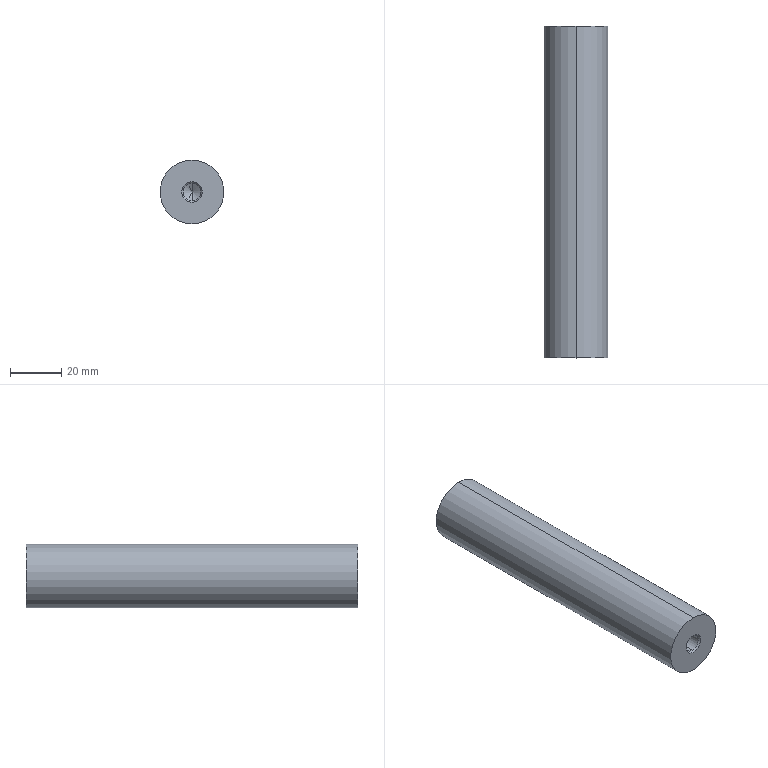Part | STEP file | A14-032 | 1 solid | 16 faces | box 25 x 130 x 25 mm | volume 62139 mm3 | cone 8 | cylinder 6 | plane 2 | commonest cylinder face diameters 6.8 x4 25 x2
STEP:
#1=CARTESIAN_POINT('',(0.,0.,0.));
#2=DIRECTION('',(0.,0.,1.));
#3=DIRECTION('',(1.,0.,0.));
#4=AXIS2_PLACEMENT_3D('',#1,#2,#3);
#5=CARTESIAN_POINT('',(0.,64.375,3.4));
#6=VERTEX_POINT('',#5);
#7=CARTESIAN_POINT('',(0.,65.,4.025));
#8=VERTEX_POINT('',#7);
#9=CARTESIAN_POINT('',(0.,65.,4.025));
#10=DIRECTION('',(0.,0.7071,0.7071));
#11=VECTOR('',#10,1.);
#12=LINE('',#9,#11);
#13=CARTESIAN_POINT('',(0.,65.,0.));
#14=DIRECTION('',(0.,1.,0.));
#15=DIRECTION('',(0.,0.,1.));
#16=AXIS2_PLACEMENT_3D('',#13,#14,#15);
#17=CONICAL_SURFACE('',#16,4.025,0.7854);
#18=CARTESIAN_POINT('',(6.283,0.));
#19=DIRECTION('',(0.,1.));
#20=VECTOR('',#19,1.);
#21=LINE('',#18,#20);
#22=(GEOMETRIC_REPRESENTATION_CONTEXT(2)PARAMETRIC_REPRESENTATION_CONTEXT()REPRESENTATION_CONTEXT('',''));
#23=DEFINITIONAL_REPRESENTATION('',(#21),#22);
#24=PCURVE('',#17,#23);
#25=CARTESIAN_POINT('',(0.,65.,0.));
#26=DIRECTION('',(0.,1.,0.));
#27=DIRECTION('',(0.,0.,1.));
#28=AXIS2_PLACEMENT_3D('',#25,#26,#27);
#29=CONICAL_SURFACE('',#28,4.025,0.7854);
#30=CARTESIAN_POINT('',(0.,0.));
#31=DIRECTION('',(0.,1.));
#32=VECTOR('',#31,1.);
#33=LINE('',#30,#32);
#34=(GEOMETRIC_REPRESENTATION_CONTEXT(2)PARAMETRIC_REPRESENTATION_CONTEXT()REPRESENTATION_CONTEXT('',''));
#35=DEFINITIONAL_REPRESENTATION('',(#33),#34);
#36=PCURVE('',#29,#35);
#37=SURFACE_CURVE('',#12,(#24,#36),.PCURVE_S1.);
#38=EDGE_CURVE('',#6,#8,#37,.T.);
#39=ORIENTED_EDGE('',*,*,#38,.T.);
#40=CARTESIAN_POINT('',(0.,65.,-4.025));
#41=VERTEX_POINT('',#40);
#42=CARTESIAN_POINT('',(0.,65.,0.));
#43=DIRECTION('',(0.,1.,0.));
#44=DIRECTION('',(0.,0.,1.));
#45=AXIS2_PLACEMENT_3D('',#42,#43,#44);
#46=CIRCLE('',#45,4.025);
#47=CARTESIAN_POINT('',(0.,0.));
#48=DIRECTION('',(1.,0.));
#49=VECTOR('',#48,1.);
#50=LINE('',#47,#49);
#51=(GEOMETRIC_REPRESENTATION_CONTEXT(2)PARAMETRIC_REPRESENTATION_CONTEXT()REPRESENTATION_CONTEXT('',''));
#52=DEFINITIONAL_REPRESENTATION('',(#50),#51);
#53=PCURVE('',#17,#52);
#54=CARTESIAN_POINT('',(0.,65.,0.));
#55=DIRECTION('',(0.,1.,0.));
#56=DIRECTION('',(0.,0.,1.));
#57=AXIS2_PLACEMENT_3D('',#54,#55,#56);
#58=PLANE('',#57);
#59=CARTESIAN_POINT('',(0.,0.));
#60=DIRECTION('',(1.,0.));
#61=AXIS2_PLACEMENT_2D('',#59,#60);
#62=CIRCLE('',#61,4.025);
#63=(GEOMETRIC_REPRESENTATION_CONTEXT(2)PARAMETRIC_REPRESENTATION_CONTEXT()REPRESENTATION_CONTEXT('',''));
#64=DEFINITIONAL_REPRESENTATION('',(#62),#63);
#65=PCURVE('',#58,#64);
#66=SURFACE_CURVE('',#46,(#53,#65),.PCURVE_S1.);
#67=EDGE_CURVE('',#41,#8,#66,.T.);
#68=ORIENTED_EDGE('',*,*,#67,.F.);
#69=CARTESIAN_POINT('',(0.,64.375,-3.4));
#70=VERTEX_POINT('',#69);
#71=CARTESIAN_POINT('',(0.,65.,-4.025));
#72=DIRECTION('',(0.,0.7071,-0.7071));
#73=VECTOR('',#72,1.);
#74=LINE('',#71,#73);
#75=CARTESIAN_POINT('',(3.142,0.));
#76=DIRECTION('',(0.,1.));
#77=VECTOR('',#76,1.);
#78=LINE('',#75,#77);
#79=(GEOMETRIC_REPRESENTATION_CONTEXT(2)PARAMETRIC_REPRESENTATION_CONTEXT()REPRESENTATION_CONTEXT('',''));
#80=DEFINITIONAL_REPRESENTATION('',(#78),#79);
#81=PCURVE('',#17,#80);
#82=CARTESIAN_POINT('',(3.142,0.));
#83=DIRECTION('',(0.,1.));
#84=VECTOR('',#83,1.);
#85=LINE('',#82,#84);
#86=(GEOMETRIC_REPRESENTATION_CONTEXT(2)PARAMETRIC_REPRESENTATION_CONTEXT()REPRESENTATION_CONTEXT('',''));
#87=DEFINITIONAL_REPRESENTATION('',(#85),#86);
#88=PCURVE('',#29,#87);
#89=SURFACE_CURVE('',#74,(#81,#88),.PCURVE_S1.);
#90=EDGE_CURVE('',#70,#41,#89,.T.);
#91=ORIENTED_EDGE('',*,*,#90,.F.);
#92=CARTESIAN_POINT('',(0.,64.375,0.));
#93=DIRECTION('',(0.,1.,0.));
#94=DIRECTION('',(0.,0.,1.));
#95=AXIS2_PLACEMENT_3D('',#92,#93,#94);
#96=CIRCLE('',#95,3.4);
#97=CARTESIAN_POINT('',(0.,-0.625));
#98=DIRECTION('',(1.,0.));
#99=VECTOR('',#98,1.);
#100=LINE('',#97,#99);
#101=(GEOMETRIC_REPRESENTATION_CONTEXT(2)PARAMETRIC_REPRESENTATION_CONTEXT()REPRESENTATION_CONTEXT('',''));
#102=DEFINITIONAL_REPRESENTATION('',(#100),#101);
#103=PCURVE('',#17,#102);
#104=CARTESIAN_POINT('',(0.,65.,0.));
#105=DIRECTION('',(0.,1.,0.));
#106=DIRECTION('',(0.,0.,1.));
#107=AXIS2_PLACEMENT_3D('',#104,#105,#106);
#108=CYLINDRICAL_SURFACE('',#107,3.4);
#109=CARTESIAN_POINT('',(0.,-0.625));
#110=DIRECTION('',(1.,0.));
#111=VECTOR('',#110,1.);
#112=LINE('',#109,#111);
#113=(GEOMETRIC_REPRESENTATION_CONTEXT(2)PARAMETRIC_REPRESENTATION_CONTEXT()REPRESENTATION_CONTEXT('',''));
#114=DEFINITIONAL_REPRESENTATION('',(#112),#113);
#115=PCURVE('',#108,#114);
#116=SURFACE_CURVE('',#96,(#103,#115),.PCURVE_S1.);
#117=EDGE_CURVE('',#70,#6,#116,.T.);
#118=ORIENTED_EDGE('',*,*,#117,.T.);
#119=EDGE_LOOP('',(#39,#68,#91,#118));
#120=FACE_BOUND('',#119,.F.);
#121=ADVANCED_FACE('',(#120),#17,.F.);
#122=CARTESIAN_POINT('',(0.,42.75,3.4));
#123=VERTEX_POINT('',#122);
#124=CARTESIAN_POINT('',(0.,65.,3.4));
#125=DIRECTION('',(0.,1.,0.));
#126=VECTOR('',#125,1.);
#127=LINE('',#124,#126);
#128=CARTESIAN_POINT('',(6.283,0.));
#129=DIRECTION('',(0.,1.));
#130=VECTOR('',#129,1.);
#131=LINE('',#128,#130);
#132=(GEOMETRIC_REPRESENTATION_CONTEXT(2)PARAMETRIC_REPRESENTATION_CONTEXT()REPRESENTATION_CONTEXT('',''));
#133=DEFINITIONAL_REPRESENTATION('',(#131),#132);
#134=PCURVE('',#108,#133);
#135=CARTESIAN_POINT('',(0.,65.,0.));
#136=DIRECTION('',(0.,1.,0.));
#137=DIRECTION('',(0.,0.,1.));
#138=AXIS2_PLACEMENT_3D('',#135,#136,#137);
#139=CYLINDRICAL_SURFACE('',#138,3.4);
#140=CARTESIAN_POINT('',(0.,0.));
#141=DIRECTION('',(0.,1.));
#142=VECTOR('',#141,1.);
#143=LINE('',#140,#142);
#144=(GEOMETRIC_REPRESENTATION_CONTEXT(2)PARAMETRIC_REPRESENTATION_CONTEXT()REPRESENTATION_CONTEXT('',''));
#145=DEFINITIONAL_REPRESENTATION('',(#143),#144);
#146=PCURVE('',#139,#145);
#147=SURFACE_CURVE('',#127,(#134,#146),.PCURVE_S1.);
#148=EDGE_CURVE('',#123,#6,#147,.T.);
#149=ORIENTED_EDGE('',*,*,#148,.T.);
#150=ORIENTED_EDGE('',*,*,#117,.F.);
#151=CARTESIAN_POINT('',(0.,42.75,-3.4));
#152=VERTEX_POINT('',#151);
#153=CARTESIAN_POINT('',(0.,65.,-3.4));
#154=DIRECTION('',(0.,1.,0.));
#155=VECTOR('',#154,1.);
#156=LINE('',#153,#155);
#157=CARTESIAN_POINT('',(3.142,0.));
#158=DIRECTION('',(0.,1.));
#159=VECTOR('',#158,1.);
#160=LINE('',#157,#159);
#161=(GEOMETRIC_REPRESENTATION_CONTEXT(2)PARAMETRIC_REPRESENTATION_CONTEXT()REPRESENTATION_CONTEXT('',''));
#162=DEFINITIONAL_REPRESENTATION('',(#160),#161);
#163=PCURVE('',#108,#162);
#164=CARTESIAN_POINT('',(3.142,0.));
#165=DIRECTION('',(0.,1.));
#166=VECTOR('',#165,1.);
#167=LINE('',#164,#166);
#168=(GEOMETRIC_REPRESENTATION_CONTEXT(2)PARAMETRIC_REPRESENTATION_CONTEXT()REPRESENTATION_CONTEXT('',''));
#169=DEFINITIONAL_REPRESENTATION('',(#167),#168);
#170=PCURVE('',#139,#169);
#171=SURFACE_CURVE('',#156,(#163,#170),.PCURVE_S1.);
#172=EDGE_CURVE('',#152,#70,#171,.T.);
#173=ORIENTED_EDGE('',*,*,#172,.F.);
#174=CARTESIAN_POINT('',(0.,42.75,0.));
#175=DIRECTION('',(0.,1.,0.));
#176=DIRECTION('',(0.,0.,1.));
#177=AXIS2_PLACEMENT_3D('',#174,#175,#176);
#178=CIRCLE('',#177,3.4);
#179=CARTESIAN_POINT('',(0.,-22.25));
#180=DIRECTION('',(1.,0.));
#181=VECTOR('',#180,1.);
#182=LINE('',#179,#181);
#183=(GEOMETRIC_REPRESENTATION_CONTEXT(2)PARAMETRIC_REPRESENTATION_CONTEXT()REPRESENTATION_CONTEXT('',''));
#184=DEFINITIONAL_REPRESENTATION('',(#182),#183);
#185=PCURVE('',#108,#184);
#186=CARTESIAN_POINT('',(0.,42.75,0.));
#187=DIRECTION('',(0.,1.,0.));
#188=DIRECTION('',(0.,0.,1.));
#189=AXIS2_PLACEMENT_3D('',#186,#187,#188);
#190=CONICAL_SURFACE('',#189,3.4,1.03);
#191=CARTESIAN_POINT('',(0.,0.));
#192=DIRECTION('',(1.,0.));
#193=VECTOR('',#192,1.);
#194=LINE('',#191,#193);
#195=(GEOMETRIC_REPRESENTATION_CONTEXT(2)PARAMETRIC_REPRESENTATION_CONTEXT()REPRESENTATION_CONTEXT('',''));
#196=DEFINITIONAL_REPRESENTATION('',(#194),#195);
#197=PCURVE('',#190,#196);
#198=SURFACE_CURVE('',#178,(#185,#197),.PCURVE_S1.);
#199=EDGE_CURVE('',#152,#123,#198,.T.);
#200=ORIENTED_EDGE('',*,*,#199,.T.);
#201=EDGE_LOOP('',(#149,#150,#173,#200));
#202=FACE_BOUND('',#201,.F.);
#203=ADVANCED_FACE('',(#202),#108,.F.);
#204=ORIENTED_EDGE('',*,*,#199,.F.);
#205=CARTESIAN_POINT('',(0.,40.707,0.));
#206=VERTEX_POINT('',#205);
#207=CARTESIAN_POINT('',(0.,42.75,-3.4));
#208=DIRECTION('',(0.,0.515,-0.8572));
#209=VECTOR('',#208,1.);
#210=LINE('',#207,#209);
#211=CARTESIAN_POINT('',(3.142,0.));
#212=DIRECTION('',(0.,1.));
#213=VECTOR('',#212,1.);
#214=LINE('',#211,#213);
#215=(GEOMETRIC_REPRESENTATION_CONTEXT(2)PARAMETRIC_REPRESENTATION_CONTEXT()REPRESENTATION_CONTEXT('',''));
#216=DEFINITIONAL_REPRESENTATION('',(#214),#215);
#217=PCURVE('',#190,#216);
#218=CARTESIAN_POINT('',(0.,42.75,0.));
#219=DIRECTION('',(0.,1.,0.));
#220=DIRECTION('',(0.,0.,1.));
#221=AXIS2_PLACEMENT_3D('',#218,#219,#220);
#222=CONICAL_SURFACE('',#221,3.4,1.03);
#223=CARTESIAN_POINT('',(3.142,0.));
#224=DIRECTION('',(0.,1.));
#225=VECTOR('',#224,1.);
#226=LINE('',#223,#225);
#227=(GEOMETRIC_REPRESENTATION_CONTEXT(2)PARAMETRIC_REPRESENTATION_CONTEXT()REPRESENTATION_CONTEXT('',''));
#228=DEFINITIONAL_REPRESENTATION('',(#226),#227);
#229=PCURVE('',#222,#228);
#230=SURFACE_CURVE('',#210,(#217,#229),.PCURVE_S1.);
#231=EDGE_CURVE('',#206,#152,#230,.T.);
#232=ORIENTED_EDGE('',*,*,#231,.F.);
#233=CARTESIAN_POINT('',(0.,42.75,3.4));
#234=DIRECTION('',(0.,0.515,0.8572));
#235=VECTOR('',#234,1.);
#236=LINE('',#233,#235);
#237=CARTESIAN_POINT('',(6.283,0.));
#238=DIRECTION('',(0.,1.));
#239=VECTOR('',#238,1.);
#240=LINE('',#237,#239);
#241=(GEOMETRIC_REPRESENTATION_CONTEXT(2)PARAMETRIC_REPRESENTATION_CONTEXT()REPRESENTATION_CONTEXT('',''));
#242=DEFINITIONAL_REPRESENTATION('',(#240),#241);
#243=PCURVE('',#190,#242);
#244=CARTESIAN_POINT('',(0.,0.));
#245=DIRECTION('',(0.,1.));
#246=VECTOR('',#245,1.);
#247=LINE('',#244,#246);
#248=(GEOMETRIC_REPRESENTATION_CONTEXT(2)PARAMETRIC_REPRESENTATION_CONTEXT()REPRESENTATION_CONTEXT('',''));
#249=DEFINITIONAL_REPRESENTATION('',(#247),#248);
#250=PCURVE('',#222,#249);
#251=SURFACE_CURVE('',#236,(#243,#250),.PCURVE_S1.);
#252=EDGE_CURVE('',#206,#123,#251,.T.);
#253=ORIENTED_EDGE('',*,*,#252,.T.);
#254=EDGE_LOOP('',(#204,#232,#253));
#255=FACE_BOUND('',#254,.F.);
#256=ADVANCED_FACE('',(#255),#190,.F.);
#257=CARTESIAN_POINT('',(0.,-64.375,-3.4));
#258=VERTEX_POINT('',#257);
#259=CARTESIAN_POINT('',(0.,-65.,-4.025));
#260=VERTEX_POINT('',#259);
#261=CARTESIAN_POINT('',(0.,-65.,-4.025));
#262=DIRECTION('',(0.,-0.7071,-0.7071));
#263=VECTOR('',#262,1.);
#264=LINE('',#261,#263);
#265=CARTESIAN_POINT('',(0.,-65.,0.));
#266=DIRECTION('',(0.,-1.,0.));
#267=DIRECTION('',(0.,0.,-1.));
#268=AXIS2_PLACEMENT_3D('',#265,#266,#267);
#269=CONICAL_SURFACE('',#268,4.025,0.7854);
#270=CARTESIAN_POINT('',(6.283,0.));
#271=DIRECTION('',(0.,1.));
#272=VECTOR('',#271,1.);
#273=LINE('',#270,#272);
#274=(GEOMETRIC_REPRESENTATION_CONTEXT(2)PARAMETRIC_REPRESENTATION_CONTEXT()REPRESENTATION_CONTEXT('',''));
#275=DEFINITIONAL_REPRESENTATION('',(#273),#274);
#276=PCURVE('',#269,#275);
#277=CARTESIAN_POINT('',(0.,-65.,0.));
#278=DIRECTION('',(0.,-1.,0.));
#279=DIRECTION('',(0.,0.,-1.));
#280=AXIS2_PLACEMENT_3D('',#277,#278,#279);
#281=CONICAL_SURFACE('',#280,4.025,0.7854);
#282=CARTESIAN_POINT('',(0.,0.));
#283=DIRECTION('',(0.,1.));
#284=VECTOR('',#283,1.);
#285=LINE('',#282,#284);
#286=(GEOMETRIC_REPRESENTATION_CONTEXT(2)PARAMETRIC_REPRESENTATION_CONTEXT()REPRESENTATION_CONTEXT('',''));
#287=DEFINITIONAL_REPRESENTATION('',(#285),#286);
#288=PCURVE('',#281,#287);
#289=SURFACE_CURVE('',#264,(#276,#288),.PCURVE_S1.);
#290=EDGE_CURVE('',#258,#260,#289,.T.);
#291=ORIENTED_EDGE('',*,*,#290,.T.);
#292=CARTESIAN_POINT('',(0.,-65.,4.025));
#293=VERTEX_POINT('',#292);
#294=CARTESIAN_POINT('',(0.,-65.,0.));
#295=DIRECTION('',(0.,-1.,0.));
#296=DIRECTION('',(0.,0.,-1.));
#297=AXIS2_PLACEMENT_3D('',#294,#295,#296);
#298=CIRCLE('',#297,4.025);
#299=CARTESIAN_POINT('',(0.,0.));
#300=DIRECTION('',(1.,0.));
#301=VECTOR('',#300,1.);
#302=LINE('',#299,#301);
#303=(GEOMETRIC_REPRESENTATION_CONTEXT(2)PARAMETRIC_REPRESENTATION_CONTEXT()REPRESENTATION_CONTEXT('',''));
#304=DEFINITIONAL_REPRESENTATION('',(#302),#303);
#305=PCURVE('',#269,#304);
#306=CARTESIAN_POINT('',(0.,-65.,0.));
#307=DIRECTION('',(0.,1.,0.));
#308=DIRECTION('',(0.,0.,1.));
#309=AXIS2_PLACEMENT_3D('',#306,#307,#308);
#310=PLANE('',#309);
#311=CARTESIAN_POINT('',(-4.025,0.));
#312=CARTESIAN_POINT('',(-4.025,6.972));
#313=CARTESIAN_POINT('',(2.013,3.486));
#314=CARTESIAN_POINT('',(8.05,0.));
#315=CARTESIAN_POINT('',(2.013,-3.486));
#316=CARTESIAN_POINT('',(-4.025,-6.972));
#317=CARTESIAN_POINT('',(-4.025,0.));
#318=(BOUNDED_CURVE()B_SPLINE_CURVE(2,(#311,#312,#313,#314,#315,#316,#317),.UNSPECIFIED.,.T.,.F.)B_SPLINE_CURVE_WITH_KNOTS((1,2,2,2,2,1),(-2.094,0.,2.094,4.189,6.283,8.378),.UNSPECIFIED.)CURVE()GEOMETRIC_REPRESENTATION_ITEM()RATIONAL_B_SPLINE_CURVE((1.,0.5,1.,0.5,1.,0.5,1.))REPRESENTATION_ITEM(''));
#319=(GEOMETRIC_REPRESENTATION_CONTEXT(2)PARAMETRIC_REPRESENTATION_CONTEXT()REPRESENTATION_CONTEXT('',''));
#320=DEFINITIONAL_REPRESENTATION('',(#318),#319);
#321=PCURVE('',#310,#320);
#322=SURFACE_CURVE('',#298,(#305,#321),.PCURVE_S1.);
#323=EDGE_CURVE('',#293,#260,#322,.T.);
#324=ORIENTED_EDGE('',*,*,#323,.F.);
#325=CARTESIAN_POINT('',(0.,-64.375,3.4));
#326=VERTEX_POINT('',#325);
#327=CARTESIAN_POINT('',(0.,-65.,4.025));
#328=DIRECTION('',(0.,-0.7071,0.7071));
#329=VECTOR('',#328,1.);
#330=LINE('',#327,#329);
#331=CARTESIAN_POINT('',(3.142,0.));
#332=DIRECTION('',(0.,1.));
#333=VECTOR('',#332,1.);
#334=LINE('',#331,#333);
#335=(GEOMETRIC_REPRESENTATION_CONTEXT(2)PARAMETRIC_REPRESENTATION_CONTEXT()REPRESENTATION_CONTEXT('',''));
#336=DEFINITIONAL_REPRESENTATION('',(#334),#335);
#337=PCURVE('',#269,#336);
#338=CARTESIAN_POINT('',(3.142,0.));
#339=DIRECTION('',(0.,1.));
#340=VECTOR('',#339,1.);
#341=LINE('',#338,#340);
#342=(GEOMETRIC_REPRESENTATION_CONTEXT(2)PARAMETRIC_REPRESENTATION_CONTEXT()REPRESENTATION_CONTEXT('',''));
#343=DEFINITIONAL_REPRESENTATION('',(#341),#342);
#344=PCURVE('',#281,#343);
#345=SURFACE_CURVE('',#330,(#337,#344),.PCURVE_S1.);
#346=EDGE_CURVE('',#326,#293,#345,.T.);
#347=ORIENTED_EDGE('',*,*,#346,.F.);
#348=CARTESIAN_POINT('',(0.,-64.375,0.));
#349=DIRECTION('',(0.,-1.,0.));
#350=DIRECTION('',(0.,0.,-1.));
#351=AXIS2_PLACEMENT_3D('',#348,#349,#350);
#352=CIRCLE('',#351,3.4);
#353=CARTESIAN_POINT('',(0.,-0.625));
#354=DIRECTION('',(1.,0.));
#355=VECTOR('',#354,1.);
#356=LINE('',#353,#355);
#357=(GEOMETRIC_REPRESENTATION_CONTEXT(2)PARAMETRIC_REPRESENTATION_CONTEXT()REPRESENTATION_CONTEXT('',''));
#358=DEFINITIONAL_REPRESENTATION('',(#356),#357);
#359=PCURVE('',#269,#358);
#360=CARTESIAN_POINT('',(0.,-65.,0.));
#361=DIRECTION('',(0.,-1.,0.));
#362=DIRECTION('',(0.,0.,-1.));
#363=AXIS2_PLACEMENT_3D('',#360,#361,#362);
#364=CYLINDRICAL_SURFACE('',#363,3.4);
#365=CARTESIAN_POINT('',(0.,-0.625));
#366=DIRECTION('',(1.,0.));
#367=VECTOR('',#366,1.);
#368=LINE('',#365,#367);
#369=(GEOMETRIC_REPRESENTATION_CONTEXT(2)PARAMETRIC_REPRESENTATION_CONTEXT()REPRESENTATION_CONTEXT('',''));
#370=DEFINITIONAL_REPRESENTATION('',(#368),#369);
#371=PCURVE('',#364,#370);
#372=SURFACE_CURVE('',#352,(#359,#371),.PCURVE_S1.);
#373=EDGE_CURVE('',#326,#258,#372,.T.);
#374=ORIENTED_EDGE('',*,*,#373,.T.);
#375=EDGE_LOOP('',(#291,#324,#347,#374));
#376=FACE_BOUND('',#375,.F.);
#377=ADVANCED_FACE('',(#376),#269,.F.);
#378=CARTESIAN_POINT('',(0.,-42.75,-3.4));
#379=VERTEX_POINT('',#378);
#380=CARTESIAN_POINT('',(0.,-65.,-3.4));
#381=DIRECTION('',(0.,-1.,0.));
#382=VECTOR('',#381,1.);
#383=LINE('',#380,#382);
#384=CARTESIAN_POINT('',(6.283,0.));
#385=DIRECTION('',(0.,1.));
#386=VECTOR('',#385,1.);
#387=LINE('',#384,#386);
#388=(GEOMETRIC_REPRESENTATION_CONTEXT(2)PARAMETRIC_REPRESENTATION_CONTEXT()REPRESENTATION_CONTEXT('',''));
#389=DEFINITIONAL_REPRESENTATION('',(#387),#388);
#390=PCURVE('',#364,#389);
#391=CARTESIAN_POINT('',(0.,-65.,0.));
#392=DIRECTION('',(0.,-1.,0.));
#393=DIRECTION('',(0.,0.,-1.));
#394=AXIS2_PLACEMENT_3D('',#391,#392,#393);
#395=CYLINDRICAL_SURFACE('',#394,3.4);
#396=CARTESIAN_POINT('',(0.,0.));
#397=DIRECTION('',(0.,1.));
#398=VECTOR('',#397,1.);
#399=LINE('',#396,#398);
#400=(GEOMETRIC_REPRESENTATION_CONTEXT(2)PARAMETRIC_REPRESENTATION_CONTEXT()REPRESENTATION_CONTEXT('',''));
#401=DEFINITIONAL_REPRESENTATION('',(#399),#400);
#402=PCURVE('',#395,#401);
#403=SURFACE_CURVE('',#383,(#390,#402),.PCURVE_S1.);
#404=EDGE_CURVE('',#379,#258,#403,.T.);
#405=ORIENTED_EDGE('',*,*,#404,.T.);
#406=ORIENTED_EDGE('',*,*,#373,.F.);
#407=CARTESIAN_POINT('',(0.,-42.75,3.4));
#408=VERTEX_POINT('',#407);
#409=CARTESIAN_POINT('',(0.,-65.,3.4));
#410=DIRECTION('',(0.,-1.,0.));
#411=VECTOR('',#410,1.);
#412=LINE('',#409,#411);
#413=CARTESIAN_POINT('',(3.142,0.));
#414=DIRECTION('',(0.,1.));
#415=VECTOR('',#414,1.);
#416=LINE('',#413,#415);
#417=(GEOMETRIC_REPRESENTATION_CONTEXT(2)PARAMETRIC_REPRESENTATION_CONTEXT()REPRESENTATION_CONTEXT('',''));
#418=DEFINITIONAL_REPRESENTATION('',(#416),#417);
#419=PCURVE('',#364,#418);
#420=CARTESIAN_POINT('',(3.142,0.));
#421=DIRECTION('',(0.,1.));
#422=VECTOR('',#421,1.);
#423=LINE('',#420,#422);
#424=(GEOMETRIC_REPRESENTATION_CONTEXT(2)PARAMETRIC_REPRESENTATION_CONTEXT()REPRESENTATION_CONTEXT('',''));
#425=DEFINITIONAL_REPRESENTATION('',(#423),#424);
#426=PCURVE('',#395,#425);
#427=SURFACE_CURVE('',#412,(#419,#426),.PCURVE_S1.);
#428=EDGE_CURVE('',#408,#326,#427,.T.);
#429=ORIENTED_EDGE('',*,*,#428,.F.);
#430=CARTESIAN_POINT('',(0.,-42.75,0.));
#431=DIRECTION('',(0.,-1.,0.));
#432=DIRECTION('',(0.,0.,-1.));
#433=AXIS2_PLACEMENT_3D('',#430,#431,#432);
#434=CIRCLE('',#433,3.4);
#435=CARTESIAN_POINT('',(0.,-22.25));
#436=DIRECTION('',(1.,0.));
#437=VECTOR('',#436,1.);
#438=LINE('',#435,#437);
#439=(GEOMETRIC_REPRESENTATION_CONTEXT(2)PARAMETRIC_REPRESENTATION_CONTEXT()REPRESENTATION_CONTEXT('',''));
#440=DEFINITIONAL_REPRESENTATION('',(#438),#439);
#441=PCURVE('',#364,#440);
#442=CARTESIAN_POINT('',(0.,-42.75,0.));
#443=DIRECTION('',(0.,-1.,0.));
#444=DIRECTION('',(0.,0.,-1.));
#445=AXIS2_PLACEMENT_3D('',#442,#443,#444);
#446=CONICAL_SURFACE('',#445,3.4,1.03);
#447=CARTESIAN_POINT('',(0.,0.));
#448=DIRECTION('',(1.,0.));
#449=VECTOR('',#448,1.);
#450=LINE('',#447,#449);
#451=(GEOMETRIC_REPRESENTATION_CONTEXT(2)PARAMETRIC_REPRESENTATION_CONTEXT()REPRESENTATION_CONTEXT('',''));
#452=DEFINITIONAL_REPRESENTATION('',(#450),#451);
#453=PCURVE('',#446,#452);
#454=SURFACE_CURVE('',#434,(#441,#453),.PCURVE_S1.);
#455=EDGE_CURVE('',#408,#379,#454,.T.);
#456=ORIENTED_EDGE('',*,*,#455,.T.);
#457=EDGE_LOOP('',(#405,#406,#429,#456));
#458=FACE_BOUND('',#457,.F.);
#459=ADVANCED_FACE('',(#458),#364,.F.);
#460=ORIENTED_EDGE('',*,*,#455,.F.);
#461=CARTESIAN_POINT('',(0.,-40.707,0.));
#462=VERTEX_POINT('',#461);
#463=CARTESIAN_POINT('',(0.,-42.75,3.4));
#464=DIRECTION('',(0.,-0.515,0.8572));
#465=VECTOR('',#464,1.);
#466=LINE('',#463,#465);
#467=CARTESIAN_POINT('',(3.142,0.));
#468=DIRECTION('',(0.,1.));
#469=VECTOR('',#468,1.);
#470=LINE('',#467,#469);
#471=(GEOMETRIC_REPRESENTATION_CONTEXT(2)PARAMETRIC_REPRESENTATION_CONTEXT()REPRESENTATION_CONTEXT('',''));
#472=DEFINITIONAL_REPRESENTATION('',(#470),#471);
#473=PCURVE('',#446,#472);
#474=CARTESIAN_POINT('',(0.,-42.75,0.));
#475=DIRECTION('',(0.,-1.,0.));
#476=DIRECTION('',(0.,0.,-1.));
#477=AXIS2_PLACEMENT_3D('',#474,#475,#476);
#478=CONICAL_SURFACE('',#477,3.4,1.03);
#479=CARTESIAN_POINT('',(3.142,0.));
#480=DIRECTION('',(0.,1.));
#481=VECTOR('',#480,1.);
#482=LINE('',#479,#481);
#483=(GEOMETRIC_REPRESENTATION_CONTEXT(2)PARAMETRIC_REPRESENTATION_CONTEXT()REPRESENTATION_CONTEXT('',''));
#484=DEFINITIONAL_REPRESENTATION('',(#482),#483);
#485=PCURVE('',#478,#484);
#486=SURFACE_CURVE('',#466,(#473,#485),.PCURVE_S1.);
#487=EDGE_CURVE('',#462,#408,#486,.T.);
#488=ORIENTED_EDGE('',*,*,#487,.F.);
#489=CARTESIAN_POINT('',(0.,-42.75,-3.4));
#490=DIRECTION('',(0.,-0.515,-0.8572));
#491=VECTOR('',#490,1.);
#492=LINE('',#489,#491);
#493=CARTESIAN_POINT('',(6.283,0.));
#494=DIRECTION('',(0.,1.));
#495=VECTOR('',#494,1.);
#496=LINE('',#493,#495);
#497=(GEOMETRIC_REPRESENTATION_CONTEXT(2)PARAMETRIC_REPRESENTATION_CONTEXT()REPRESENTATION_CONTEXT('',''));
#498=DEFINITIONAL_REPRESENTATION('',(#496),#497);
#499=PCURVE('',#446,#498);
#500=CARTESIAN_POINT('',(0.,0.));
#501=DIRECTION('',(0.,1.));
#502=VECTOR('',#501,1.);
#503=LINE('',#500,#502);
#504=(GEOMETRIC_REPRESENTATION_CONTEXT(2)PARAMETRIC_REPRESENTATION_CONTEXT()REPRESENTATION_CONTEXT('',''));
#505=DEFINITIONAL_REPRESENTATION('',(#503),#504);
#506=PCURVE('',#478,#505);
#507=SURFACE_CURVE('',#492,(#499,#506),.PCURVE_S1.);
#508=EDGE_CURVE('',#462,#379,#507,.T.);
#509=ORIENTED_EDGE('',*,*,#508,.T.);
#510=EDGE_LOOP('',(#460,#488,#509));
#511=FACE_BOUND('',#510,.F.);
#512=ADVANCED_FACE('',(#511),#446,.F.);
#513=CARTESIAN_POINT('',(0.,65.,12.5));
#514=VERTEX_POINT('',#513);
#515=CARTESIAN_POINT('',(0.,65.,-12.5));
#516=VERTEX_POINT('',#515);
#517=CARTESIAN_POINT('',(0.,65.,0.));
#518=DIRECTION('',(0.,1.,0.));
#519=DIRECTION('',(0.,0.,1.));
#520=AXIS2_PLACEMENT_3D('',#517,#518,#519);
#521=CIRCLE('',#520,12.5);
#522=CARTESIAN_POINT('',(0.,65.,0.));
#523=DIRECTION('',(0.,-1.,0.));
#524=DIRECTION('',(0.,0.,-1.));
#525=AXIS2_PLACEMENT_3D('',#522,#523,#524);
#526=CYLINDRICAL_SURFACE('',#525,12.5);
#527=CARTESIAN_POINT('',(3.142,0.));
#528=DIRECTION('',(-1.,0.));
#529=VECTOR('',#528,1.);
#530=LINE('',#527,#529);
#531=(GEOMETRIC_REPRESENTATION_CONTEXT(2)PARAMETRIC_REPRESENTATION_CONTEXT()REPRESENTATION_CONTEXT('',''));
#532=DEFINITIONAL_REPRESENTATION('',(#530),#531);
#533=PCURVE('',#526,#532);
#534=CARTESIAN_POINT('',(0.,0.));
#535=DIRECTION('',(1.,0.));
#536=AXIS2_PLACEMENT_2D('',#534,#535);
#537=CIRCLE('',#536,12.5);
#538=(GEOMETRIC_REPRESENTATION_CONTEXT(2)PARAMETRIC_REPRESENTATION_CONTEXT()REPRESENTATION_CONTEXT('',''));
#539=DEFINITIONAL_REPRESENTATION('',(#537),#538);
#540=PCURVE('',#58,#539);
#541=SURFACE_CURVE('',#521,(#533,#540),.PCURVE_S1.);
#542=EDGE_CURVE('',#514,#516,#541,.T.);
#543=ORIENTED_EDGE('',*,*,#542,.F.);
#544=CARTESIAN_POINT('',(0.,-65.,12.5));
#545=VERTEX_POINT('',#544);
#546=CARTESIAN_POINT('',(0.,65.,12.5));
#547=DIRECTION('',(0.,-1.,0.));
#548=VECTOR('',#547,1.);
#549=LINE('',#546,#548);
#550=CARTESIAN_POINT('',(3.142,0.));
#551=DIRECTION('',(0.,1.));
#552=VECTOR('',#551,1.);
#553=LINE('',#550,#552);
#554=(GEOMETRIC_REPRESENTATION_CONTEXT(2)PARAMETRIC_REPRESENTATION_CONTEXT()REPRESENTATION_CONTEXT('',''));
#555=DEFINITIONAL_REPRESENTATION('',(#553),#554);
#556=PCURVE('',#526,#555);
#557=CARTESIAN_POINT('',(0.,65.,0.));
#558=DIRECTION('',(0.,-1.,0.));
#559=DIRECTION('',(0.,0.,-1.));
#560=AXIS2_PLACEMENT_3D('',#557,#558,#559);
#561=CYLINDRICAL_SURFACE('',#560,12.5);
#562=CARTESIAN_POINT('',(3.142,0.));
#563=DIRECTION('',(0.,1.));
#564=VECTOR('',#563,1.);
#565=LINE('',#562,#564);
#566=(GEOMETRIC_REPRESENTATION_CONTEXT(2)PARAMETRIC_REPRESENTATION_CONTEXT()REPRESENTATION_CONTEXT('',''));
#567=DEFINITIONAL_REPRESENTATION('',(#565),#566);
#568=PCURVE('',#561,#567);
#569=SURFACE_CURVE('',#549,(#556,#568),.PCURVE_S1.);
#570=EDGE_CURVE('',#514,#545,#569,.T.);
#571=ORIENTED_EDGE('',*,*,#570,.T.);
#572=CARTESIAN_POINT('',(0.,-65.,-12.5));
#573=VERTEX_POINT('',#572);
#574=CARTESIAN_POINT('',(0.,-65.,0.));
#575=DIRECTION('',(0.,1.,0.));
#576=DIRECTION('',(0.,0.,1.));
#577=AXIS2_PLACEMENT_3D('',#574,#575,#576);
#578=CIRCLE('',#577,12.5);
#579=CARTESIAN_POINT('',(3.142,130.));
#580=DIRECTION('',(-1.,0.));
#581=VECTOR('',#580,1.);
#582=LINE('',#579,#581);
#583=(GEOMETRIC_REPRESENTATION_CONTEXT(2)PARAMETRIC_REPRESENTATION_CONTEXT()REPRESENTATION_CONTEXT('',''));
#584=DEFINITIONAL_REPRESENTATION('',(#582),#583);
#585=PCURVE('',#526,#584);
#586=CARTESIAN_POINT('',(0.,0.));
#587=DIRECTION('',(1.,0.));
#588=AXIS2_PLACEMENT_2D('',#586,#587);
#589=CIRCLE('',#588,12.5);
#590=(GEOMETRIC_REPRESENTATION_CONTEXT(2)PARAMETRIC_REPRESENTATION_CONTEXT()REPRESENTATION_CONTEXT('',''));
#591=DEFINITIONAL_REPRESENTATION('',(#589),#590);
#592=PCURVE('',#310,#591);
#593=SURFACE_CURVE('',#578,(#585,#592),.PCURVE_S1.);
#594=EDGE_CURVE('',#545,#573,#593,.T.);
#595=ORIENTED_EDGE('',*,*,#594,.T.);
#596=CARTESIAN_POINT('',(0.,65.,-12.5));
#597=DIRECTION('',(0.,-1.,0.));
#598=VECTOR('',#597,1.);
#599=LINE('',#596,#598);
#600=CARTESIAN_POINT('',(0.,0.));
#601=DIRECTION('',(0.,1.));
#602=VECTOR('',#601,1.);
#603=LINE('',#600,#602);
#604=(GEOMETRIC_REPRESENTATION_CONTEXT(2)PARAMETRIC_REPRESENTATION_CONTEXT()REPRESENTATION_CONTEXT('',''));
#605=DEFINITIONAL_REPRESENTATION('',(#603),#604);
#606=PCURVE('',#526,#605);
#607=CARTESIAN_POINT('',(6.283,0.));
#608=DIRECTION('',(0.,1.));
#609=VECTOR('',#608,1.);
#610=LINE('',#607,#609);
#611=(GEOMETRIC_REPRESENTATION_CONTEXT(2)PARAMETRIC_REPRESENTATION_CONTEXT()REPRESENTATION_CONTEXT('',''));
#612=DEFINITIONAL_REPRESENTATION('',(#610),#611);
#613=PCURVE('',#561,#612);
#614=SURFACE_CURVE('',#599,(#606,#613),.PCURVE_S1.);
#615=EDGE_CURVE('',#516,#573,#614,.T.);
#616=ORIENTED_EDGE('',*,*,#615,.F.);
#617=EDGE_LOOP('',(#543,#571,#595,#616));
#618=FACE_BOUND('',#617,.T.);
#619=ADVANCED_FACE('',(#618),#526,.T.);
#620=ORIENTED_EDGE('',*,*,#570,.F.);
#621=CARTESIAN_POINT('',(0.,65.,0.));
#622=DIRECTION('',(0.,1.,0.));
#623=DIRECTION('',(0.,0.,1.));
#624=AXIS2_PLACEMENT_3D('',#621,#622,#623);
#625=CIRCLE('',#624,12.5);
#626=CARTESIAN_POINT('',(9.425,0.));
#627=DIRECTION('',(-1.,0.));
#628=VECTOR('',#627,1.);
#629=LINE('',#626,#628);
#630=(GEOMETRIC_REPRESENTATION_CONTEXT(2)PARAMETRIC_REPRESENTATION_CONTEXT()REPRESENTATION_CONTEXT('',''));
#631=DEFINITIONAL_REPRESENTATION('',(#629),#630);
#632=PCURVE('',#561,#631);
#633=CARTESIAN_POINT('',(0.,0.));
#634=DIRECTION('',(1.,0.));
#635=AXIS2_PLACEMENT_2D('',#633,#634);
#636=CIRCLE('',#635,12.5);
#637=(GEOMETRIC_REPRESENTATION_CONTEXT(2)PARAMETRIC_REPRESENTATION_CONTEXT()REPRESENTATION_CONTEXT('',''));
#638=DEFINITIONAL_REPRESENTATION('',(#636),#637);
#639=PCURVE('',#58,#638);
#640=SURFACE_CURVE('',#625,(#632,#639),.PCURVE_S1.);
#641=EDGE_CURVE('',#516,#514,#640,.T.);
#642=ORIENTED_EDGE('',*,*,#641,.F.);
#643=ORIENTED_EDGE('',*,*,#615,.T.);
#644=CARTESIAN_POINT('',(0.,-65.,0.));
#645=DIRECTION('',(0.,1.,0.));
#646=DIRECTION('',(0.,0.,1.));
#647=AXIS2_PLACEMENT_3D('',#644,#645,#646);
#648=CIRCLE('',#647,12.5);
#649=CARTESIAN_POINT('',(9.425,130.));
#650=DIRECTION('',(-1.,0.));
#651=VECTOR('',#650,1.);
#652=LINE('',#649,#651);
#653=(GEOMETRIC_REPRESENTATION_CONTEXT(2)PARAMETRIC_REPRESENTATION_CONTEXT()REPRESENTATION_CONTEXT('',''));
#654=DEFINITIONAL_REPRESENTATION('',(#652),#653);
#655=PCURVE('',#561,#654);
#656=CARTESIAN_POINT('',(0.,0.));
#657=DIRECTION('',(1.,0.));
#658=AXIS2_PLACEMENT_2D('',#656,#657);
#659=CIRCLE('',#658,12.5);
#660=(GEOMETRIC_REPRESENTATION_CONTEXT(2)PARAMETRIC_REPRESENTATION_CONTEXT()REPRESENTATION_CONTEXT('',''));
#661=DEFINITIONAL_REPRESENTATION('',(#659),#660);
#662=PCURVE('',#310,#661);
#663=SURFACE_CURVE('',#648,(#655,#662),.PCURVE_S1.);
#664=EDGE_CURVE('',#573,#545,#663,.T.);
#665=ORIENTED_EDGE('',*,*,#664,.T.);
#666=EDGE_LOOP('',(#620,#642,#643,#665));
#667=FACE_BOUND('',#666,.T.);
#668=ADVANCED_FACE('',(#667),#561,.T.);
#669=CARTESIAN_POINT('',(0.,65.,0.));
#670=DIRECTION('',(0.,1.,0.));
#671=DIRECTION('',(0.,0.,1.));
#672=AXIS2_PLACEMENT_3D('',#669,#670,#671);
#673=CIRCLE('',#672,4.025);
#674=CARTESIAN_POINT('',(0.,0.));
#675=DIRECTION('',(1.,0.));
#676=AXIS2_PLACEMENT_2D('',#674,#675);
#677=CIRCLE('',#676,4.025);
#678=(GEOMETRIC_REPRESENTATION_CONTEXT(2)PARAMETRIC_REPRESENTATION_CONTEXT()REPRESENTATION_CONTEXT('',''));
#679=DEFINITIONAL_REPRESENTATION('',(#677),#678);
#680=PCURVE('',#58,#679);
#681=CARTESIAN_POINT('',(0.,0.));
#682=DIRECTION('',(1.,0.));
#683=VECTOR('',#682,1.);
#684=LINE('',#681,#683);
#685=(GEOMETRIC_REPRESENTATION_CONTEXT(2)PARAMETRIC_REPRESENTATION_CONTEXT()REPRESENTATION_CONTEXT('',''));
#686=DEFINITIONAL_REPRESENTATION('',(#684),#685);
#687=PCURVE('',#29,#686);
#688=SURFACE_CURVE('',#673,(#680,#687),.PCURVE_S1.);
#689=EDGE_CURVE('',#8,#41,#688,.T.);
#690=ORIENTED_EDGE('',*,*,#689,.F.);
#691=ORIENTED_EDGE('',*,*,#67,.F.);
#692=EDGE_LOOP('',(#690,#691));
#693=FACE_BOUND('',#692,.T.);
#694=ORIENTED_EDGE('',*,*,#641,.T.);
#695=ORIENTED_EDGE('',*,*,#542,.T.);
#696=EDGE_LOOP('',(#694,#695));
#697=FACE_BOUND('',#696,.T.);
#698=ADVANCED_FACE('',(#693,#697),#58,.T.);
#699=CARTESIAN_POINT('',(0.,-65.,0.));
#700=DIRECTION('',(0.,-1.,0.));
#701=DIRECTION('',(0.,0.,-1.));
#702=AXIS2_PLACEMENT_3D('',#699,#700,#701);
#703=CIRCLE('',#702,4.025);
#704=CARTESIAN_POINT('',(-4.025,0.));
#705=CARTESIAN_POINT('',(-4.025,6.972));
#706=CARTESIAN_POINT('',(2.013,3.486));
#707=CARTESIAN_POINT('',(8.05,0.));
#708=CARTESIAN_POINT('',(2.013,-3.486));
#709=CARTESIAN_POINT('',(-4.025,-6.972));
#710=CARTESIAN_POINT('',(-4.025,0.));
#711=(BOUNDED_CURVE()B_SPLINE_CURVE(2,(#704,#705,#706,#707,#708,#709,#710),.UNSPECIFIED.,.T.,.F.)B_SPLINE_CURVE_WITH_KNOTS((1,2,2,2,2,1),(-2.094,0.,2.094,4.189,6.283,8.378),.UNSPECIFIED.)CURVE()GEOMETRIC_REPRESENTATION_ITEM()RATIONAL_B_SPLINE_CURVE((1.,0.5,1.,0.5,1.,0.5,1.))REPRESENTATION_ITEM(''));
#712=(GEOMETRIC_REPRESENTATION_CONTEXT(2)PARAMETRIC_REPRESENTATION_CONTEXT()REPRESENTATION_CONTEXT('',''));
#713=DEFINITIONAL_REPRESENTATION('',(#711),#712);
#714=PCURVE('',#310,#713);
#715=CARTESIAN_POINT('',(0.,0.));
#716=DIRECTION('',(1.,0.));
#717=VECTOR('',#716,1.);
#718=LINE('',#715,#717);
#719=(GEOMETRIC_REPRESENTATION_CONTEXT(2)PARAMETRIC_REPRESENTATION_CONTEXT()REPRESENTATION_CONTEXT('',''));
#720=DEFINITIONAL_REPRESENTATION('',(#718),#719);
#721=PCURVE('',#281,#720);
#722=SURFACE_CURVE('',#703,(#714,#721),.PCURVE_S1.);
#723=EDGE_CURVE('',#260,#293,#722,.T.);
#724=ORIENTED_EDGE('',*,*,#723,.F.);
#725=ORIENTED_EDGE('',*,*,#323,.F.);
#726=EDGE_LOOP('',(#724,#725));
#727=FACE_BOUND('',#726,.T.);
#728=ORIENTED_EDGE('',*,*,#664,.F.);
#729=ORIENTED_EDGE('',*,*,#594,.F.);
#730=EDGE_LOOP('',(#728,#729));
#731=FACE_BOUND('',#730,.T.);
#732=ADVANCED_FACE('',(#727,#731),#310,.F.);
#733=CARTESIAN_POINT('',(0.,-42.75,0.));
#734=DIRECTION('',(0.,-1.,0.));
#735=DIRECTION('',(0.,0.,-1.));
#736=AXIS2_PLACEMENT_3D('',#733,#734,#735);
#737=CIRCLE('',#736,3.4);
#738=CARTESIAN_POINT('',(0.,0.));
#739=DIRECTION('',(1.,0.));
#740=VECTOR('',#739,1.);
#741=LINE('',#738,#740);
#742=(GEOMETRIC_REPRESENTATION_CONTEXT(2)PARAMETRIC_REPRESENTATION_CONTEXT()REPRESENTATION_CONTEXT('',''));
#743=DEFINITIONAL_REPRESENTATION('',(#741),#742);
#744=PCURVE('',#478,#743);
#745=CARTESIAN_POINT('',(0.,-22.25));
#746=DIRECTION('',(1.,0.));
#747=VECTOR('',#746,1.);
#748=LINE('',#745,#747);
#749=(GEOMETRIC_REPRESENTATION_CONTEXT(2)PARAMETRIC_REPRESENTATION_CONTEXT()REPRESENTATION_CONTEXT('',''));
#750=DEFINITIONAL_REPRESENTATION('',(#748),#749);
#751=PCURVE('',#395,#750);
#752=SURFACE_CURVE('',#737,(#744,#751),.PCURVE_S1.);
#753=EDGE_CURVE('',#379,#408,#752,.T.);
#754=ORIENTED_EDGE('',*,*,#753,.F.);
#755=ORIENTED_EDGE('',*,*,#508,.F.);
#756=ORIENTED_EDGE('',*,*,#487,.T.);
#757=EDGE_LOOP('',(#754,#755,#756));
#758=FACE_BOUND('',#757,.F.);
#759=ADVANCED_FACE('',(#758),#478,.F.);
#760=CARTESIAN_POINT('',(0.,-64.375,0.));
#761=DIRECTION('',(0.,-1.,0.));
#762=DIRECTION('',(0.,0.,-1.));
#763=AXIS2_PLACEMENT_3D('',#760,#761,#762);
#764=CIRCLE('',#763,3.4);
#765=CARTESIAN_POINT('',(0.,-0.625));
#766=DIRECTION('',(1.,0.));
#767=VECTOR('',#766,1.);
#768=LINE('',#765,#767);
#769=(GEOMETRIC_REPRESENTATION_CONTEXT(2)PARAMETRIC_REPRESENTATION_CONTEXT()REPRESENTATION_CONTEXT('',''));
#770=DEFINITIONAL_REPRESENTATION('',(#768),#769);
#771=PCURVE('',#395,#770);
#772=CARTESIAN_POINT('',(0.,-0.625));
#773=DIRECTION('',(1.,0.));
#774=VECTOR('',#773,1.);
#775=LINE('',#772,#774);
#776=(GEOMETRIC_REPRESENTATION_CONTEXT(2)PARAMETRIC_REPRESENTATION_CONTEXT()REPRESENTATION_CONTEXT('',''));
#777=DEFINITIONAL_REPRESENTATION('',(#775),#776);
#778=PCURVE('',#281,#777);
#779=SURFACE_CURVE('',#764,(#771,#778),.PCURVE_S1.);
#780=EDGE_CURVE('',#258,#326,#779,.T.);
#781=ORIENTED_EDGE('',*,*,#780,.F.);
#782=ORIENTED_EDGE('',*,*,#404,.F.);
#783=ORIENTED_EDGE('',*,*,#753,.T.);
#784=ORIENTED_EDGE('',*,*,#428,.T.);
#785=EDGE_LOOP('',(#781,#782,#783,#784));
#786=FACE_BOUND('',#785,.F.);
#787=ADVANCED_FACE('',(#786),#395,.F.);
#788=ORIENTED_EDGE('',*,*,#723,.F.);
#789=ORIENTED_EDGE('',*,*,#290,.F.);
#790=ORIENTED_EDGE('',*,*,#780,.T.);
#791=ORIENTED_EDGE('',*,*,#346,.T.);
#792=EDGE_LOOP('',(#788,#789,#790,#791));
#793=FACE_BOUND('',#792,.F.);
#794=ADVANCED_FACE('',(#793),#281,.F.);
#795=CARTESIAN_POINT('',(0.,42.75,0.));
#796=DIRECTION('',(0.,1.,0.));
#797=DIRECTION('',(0.,0.,1.));
#798=AXIS2_PLACEMENT_3D('',#795,#796,#797);
#799=CIRCLE('',#798,3.4);
#800=CARTESIAN_POINT('',(0.,0.));
#801=DIRECTION('',(1.,0.));
#802=VECTOR('',#801,1.);
#803=LINE('',#800,#802);
#804=(GEOMETRIC_REPRESENTATION_CONTEXT(2)PARAMETRIC_REPRESENTATION_CONTEXT()REPRESENTATION_CONTEXT('',''));
#805=DEFINITIONAL_REPRESENTATION('',(#803),#804);
#806=PCURVE('',#222,#805);
#807=CARTESIAN_POINT('',(0.,-22.25));
#808=DIRECTION('',(1.,0.));
#809=VECTOR('',#808,1.);
#810=LINE('',#807,#809);
#811=(GEOMETRIC_REPRESENTATION_CONTEXT(2)PARAMETRIC_REPRESENTATION_CONTEXT()REPRESENTATION_CONTEXT('',''));
#812=DEFINITIONAL_REPRESENTATION('',(#810),#811);
#813=PCURVE('',#139,#812);
#814=SURFACE_CURVE('',#799,(#806,#813),.PCURVE_S1.);
#815=EDGE_CURVE('',#123,#152,#814,.T.);
#816=ORIENTED_EDGE('',*,*,#815,.F.);
#817=ORIENTED_EDGE('',*,*,#252,.F.);
#818=ORIENTED_EDGE('',*,*,#231,.T.);
#819=EDGE_LOOP('',(#816,#817,#818));
#820=FACE_BOUND('',#819,.F.);
#821=ADVANCED_FACE('',(#820),#222,.F.);
#822=CARTESIAN_POINT('',(0.,64.375,0.));
#823=DIRECTION('',(0.,1.,0.));
#824=DIRECTION('',(0.,0.,1.));
#825=AXIS2_PLACEMENT_3D('',#822,#823,#824);
#826=CIRCLE('',#825,3.4);
#827=CARTESIAN_POINT('',(0.,-0.625));
#828=DIRECTION('',(1.,0.));
#829=VECTOR('',#828,1.);
#830=LINE('',#827,#829);
#831=(GEOMETRIC_REPRESENTATION_CONTEXT(2)PARAMETRIC_REPRESENTATION_CONTEXT()REPRESENTATION_CONTEXT('',''));
#832=DEFINITIONAL_REPRESENTATION('',(#830),#831);
#833=PCURVE('',#139,#832);
#834=CARTESIAN_POINT('',(0.,-0.625));
#835=DIRECTION('',(1.,0.));
#836=VECTOR('',#835,1.);
#837=LINE('',#834,#836);
#838=(GEOMETRIC_REPRESENTATION_CONTEXT(2)PARAMETRIC_REPRESENTATION_CONTEXT()REPRESENTATION_CONTEXT('',''));
#839=DEFINITIONAL_REPRESENTATION('',(#837),#838);
#840=PCURVE('',#29,#839);
#841=SURFACE_CURVE('',#826,(#833,#840),.PCURVE_S1.);
#842=EDGE_CURVE('',#6,#70,#841,.T.);
#843=ORIENTED_EDGE('',*,*,#842,.F.);
#844=ORIENTED_EDGE('',*,*,#148,.F.);
#845=ORIENTED_EDGE('',*,*,#815,.T.);
#846=ORIENTED_EDGE('',*,*,#172,.T.);
#847=EDGE_LOOP('',(#843,#844,#845,#846));
#848=FACE_BOUND('',#847,.F.);
#849=ADVANCED_FACE('',(#848),#139,.F.);
#850=ORIENTED_EDGE('',*,*,#689,.F.);
#851=ORIENTED_EDGE('',*,*,#38,.F.);
#852=ORIENTED_EDGE('',*,*,#842,.T.);
#853=ORIENTED_EDGE('',*,*,#90,.T.);
#854=EDGE_LOOP('',(#850,#851,#852,#853));
#855=FACE_BOUND('',#854,.F.);
#856=ADVANCED_FACE('',(#855),#29,.F.);
#857=CLOSED_SHELL('',(#121,#203,#256,#377,#459,#512,#619,#668,#698,#732,#759,#787,#794,#821,#849,#856));
#858=MANIFOLD_SOLID_BREP('',#857);
#859=(LENGTH_UNIT()NAMED_UNIT(*)SI_UNIT(.MILLI.,.METRE.));
#860=UNCERTAINTY_MEASURE_WITH_UNIT(LENGTH_MEASURE(0.0000001),#859,'','');
#861=(NAMED_UNIT(*)PLANE_ANGLE_UNIT()SI_UNIT($,.RADIAN.));
#862=(NAMED_UNIT(*)SI_UNIT($,.STERADIAN.)SOLID_ANGLE_UNIT());
#863=(GEOMETRIC_REPRESENTATION_CONTEXT(3)GLOBAL_UNCERTAINTY_ASSIGNED_CONTEXT((#860))GLOBAL_UNIT_ASSIGNED_CONTEXT((#859,#861,#862))REPRESENTATION_CONTEXT('',''));
#864=ADVANCED_BREP_SHAPE_REPRESENTATION('',(#4,#858),#863);